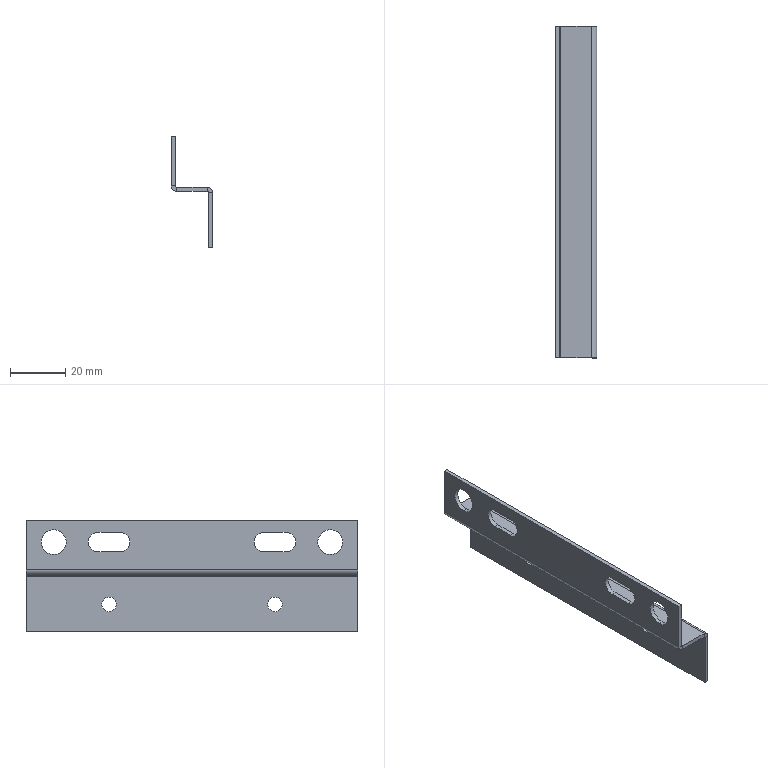Part | STEP file | 1 solid | 38 faces | box 15 x 120 x 40.5 mm | volume 8986 mm3 | plane 22 | cylinder 16 | commonest cylinder face diameters 5.3 x4 7 x4 9 x4 1 x2 4 x2